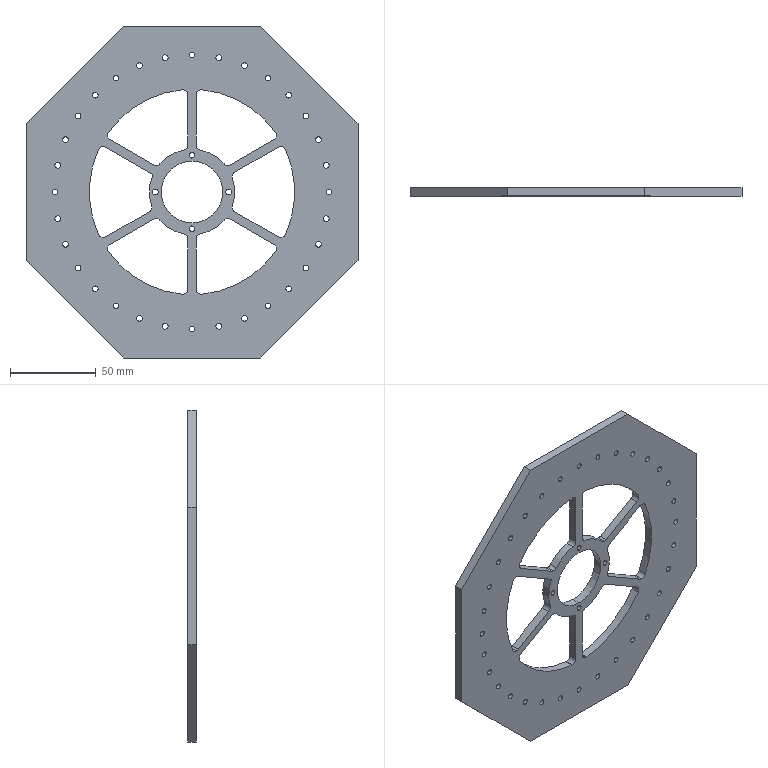Part | SolidWorks | features ICE 7, CirPattern 4, Extrusion 1, Fillet 1 | 1 solid | 137 faces | box 194.015 x 5 x 194.015 mm | volume 108020 mm3 | cylinder 115 | plane 22 | commonest cylinder face diameters 3.3 x72 6 x29 50 x6 120 x6 36 x2